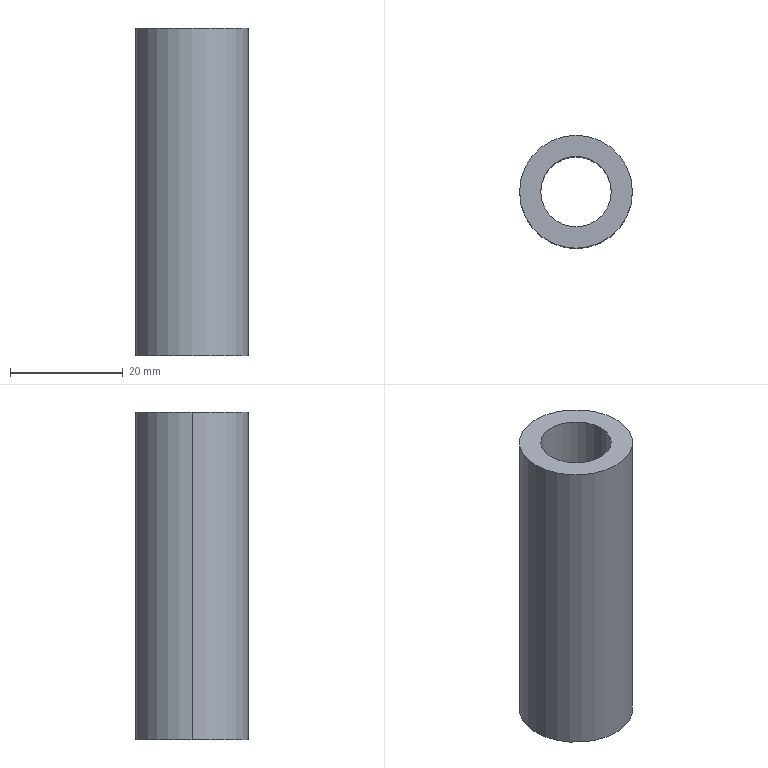Part | STEP file | X77-08309 | 1 solid | 6 faces | box 20 x 20 x 58 mm | volume 11104 mm3 | cylinder 4 | plane 2 | commonest cylinder face diameters 12.5 x2 20 x2
STEP:
#1=CARTESIAN_POINT('',(-36.25,627.253,58.));
#2=VERTEX_POINT('',#1);
#3=CARTESIAN_POINT('',(-23.75,627.253,58.));
#4=VERTEX_POINT('',#3);
#5=CARTESIAN_POINT('',(-30.,627.253,58.));
#6=DIRECTION('',(0.,0.,1.));
#7=DIRECTION('',(1.,0.,0.));
#8=AXIS2_PLACEMENT_3D('',#5,#6,#7);
#9=CIRCLE('',#8,6.25);
#10=EDGE_CURVE('',#2,#4,#9,.T.);
#11=ORIENTED_EDGE('',*,*,#10,.T.);
#12=CARTESIAN_POINT('',(-23.75,627.253,0.));
#13=VERTEX_POINT('',#12);
#14=CARTESIAN_POINT('',(-23.75,627.253,58.));
#15=DIRECTION('',(0.,0.,-1.));
#16=VECTOR('',#15,1000.);
#17=LINE('',#14,#16);
#18=EDGE_CURVE('',#4,#13,#17,.T.);
#19=ORIENTED_EDGE('',*,*,#18,.T.);
#20=CARTESIAN_POINT('',(-36.25,627.253,0.));
#21=VERTEX_POINT('',#20);
#22=CARTESIAN_POINT('',(-30.,627.253,0.));
#23=DIRECTION('',(0.,0.,1.));
#24=DIRECTION('',(1.,0.,0.));
#25=AXIS2_PLACEMENT_3D('',#22,#23,#24);
#26=CIRCLE('',#25,6.25);
#27=EDGE_CURVE('',#21,#13,#26,.T.);
#28=ORIENTED_EDGE('',*,*,#27,.F.);
#29=CARTESIAN_POINT('',(-36.25,627.253,58.));
#30=DIRECTION('',(0.,0.,-1.));
#31=VECTOR('',#30,1000.);
#32=LINE('',#29,#31);
#33=EDGE_CURVE('',#2,#21,#32,.T.);
#34=ORIENTED_EDGE('',*,*,#33,.F.);
#35=EDGE_LOOP('',(#11,#19,#28,#34));
#36=FACE_OUTER_BOUND('',#35,.T.);
#37=CARTESIAN_POINT('',(-30.,627.253,58.));
#38=DIRECTION('',(0.,0.,-1.));
#39=DIRECTION('',(-1.,0.,0.));
#40=AXIS2_PLACEMENT_3D('',#37,#38,#39);
#41=CYLINDRICAL_SURFACE('',#40,6.25);
#42=ADVANCED_FACE('',(#36),#41,.F.);
#43=CARTESIAN_POINT('',(-20.,627.253,58.));
#44=VERTEX_POINT('',#43);
#45=CARTESIAN_POINT('',(-40.,627.253,58.));
#46=VERTEX_POINT('',#45);
#47=CARTESIAN_POINT('',(-30.,627.253,58.));
#48=DIRECTION('',(0.,0.,1.));
#49=DIRECTION('',(1.,0.,0.));
#50=AXIS2_PLACEMENT_3D('',#47,#48,#49);
#51=CIRCLE('',#50,10.);
#52=EDGE_CURVE('',#44,#46,#51,.T.);
#53=ORIENTED_EDGE('',*,*,#52,.F.);
#54=CARTESIAN_POINT('',(-20.,627.253,0.));
#55=VERTEX_POINT('',#54);
#56=CARTESIAN_POINT('',(-20.,627.253,58.));
#57=DIRECTION('',(0.,0.,-1.));
#58=VECTOR('',#57,1000.);
#59=LINE('',#56,#58);
#60=EDGE_CURVE('',#44,#55,#59,.T.);
#61=ORIENTED_EDGE('',*,*,#60,.T.);
#62=CARTESIAN_POINT('',(-40.,627.253,0.));
#63=VERTEX_POINT('',#62);
#64=CARTESIAN_POINT('',(-30.,627.253,0.));
#65=DIRECTION('',(0.,0.,1.));
#66=DIRECTION('',(1.,0.,0.));
#67=AXIS2_PLACEMENT_3D('',#64,#65,#66);
#68=CIRCLE('',#67,10.);
#69=EDGE_CURVE('',#55,#63,#68,.T.);
#70=ORIENTED_EDGE('',*,*,#69,.T.);
#71=CARTESIAN_POINT('',(-40.,627.253,58.));
#72=DIRECTION('',(0.,0.,-1.));
#73=VECTOR('',#72,1000.);
#74=LINE('',#71,#73);
#75=EDGE_CURVE('',#46,#63,#74,.T.);
#76=ORIENTED_EDGE('',*,*,#75,.F.);
#77=EDGE_LOOP('',(#53,#61,#70,#76));
#78=FACE_OUTER_BOUND('',#77,.T.);
#79=CARTESIAN_POINT('',(-30.,627.253,58.));
#80=DIRECTION('',(0.,0.,-1.));
#81=DIRECTION('',(-1.,0.,0.));
#82=AXIS2_PLACEMENT_3D('',#79,#80,#81);
#83=CYLINDRICAL_SURFACE('',#82,10.);
#84=ADVANCED_FACE('',(#78),#83,.T.);
#85=CARTESIAN_POINT('',(-30.,627.253,58.));
#86=DIRECTION('',(0.,0.,1.));
#87=DIRECTION('',(1.,0.,0.));
#88=AXIS2_PLACEMENT_3D('',#85,#86,#87);
#89=CIRCLE('',#88,10.);
#90=EDGE_CURVE('',#46,#44,#89,.T.);
#91=ORIENTED_EDGE('',*,*,#90,.T.);
#92=ORIENTED_EDGE('',*,*,#52,.T.);
#93=EDGE_LOOP('',(#91,#92));
#94=FACE_OUTER_BOUND('',#93,.T.);
#95=ORIENTED_EDGE('',*,*,#10,.F.);
#96=CARTESIAN_POINT('',(-30.,627.253,58.));
#97=DIRECTION('',(0.,0.,1.));
#98=DIRECTION('',(1.,0.,0.));
#99=AXIS2_PLACEMENT_3D('',#96,#97,#98);
#100=CIRCLE('',#99,6.25);
#101=EDGE_CURVE('',#4,#2,#100,.T.);
#102=ORIENTED_EDGE('',*,*,#101,.F.);
#103=EDGE_LOOP('',(#95,#102));
#104=FACE_BOUND('',#103,.T.);
#105=CARTESIAN_POINT('',(-30.,627.253,58.));
#106=DIRECTION('',(0.,0.,1.));
#107=DIRECTION('',(1.,0.,0.));
#108=AXIS2_PLACEMENT_3D('',#105,#106,#107);
#109=PLANE('',#108);
#110=ADVANCED_FACE('',(#94,#104),#109,.T.);
#111=CARTESIAN_POINT('',(-30.,627.253,0.));
#112=DIRECTION('',(0.,0.,1.));
#113=DIRECTION('',(1.,0.,0.));
#114=AXIS2_PLACEMENT_3D('',#111,#112,#113);
#115=CIRCLE('',#114,10.);
#116=EDGE_CURVE('',#63,#55,#115,.T.);
#117=ORIENTED_EDGE('',*,*,#116,.F.);
#118=ORIENTED_EDGE('',*,*,#69,.F.);
#119=EDGE_LOOP('',(#117,#118));
#120=FACE_OUTER_BOUND('',#119,.T.);
#121=ORIENTED_EDGE('',*,*,#27,.T.);
#122=CARTESIAN_POINT('',(-30.,627.253,0.));
#123=DIRECTION('',(0.,0.,1.));
#124=DIRECTION('',(1.,0.,0.));
#125=AXIS2_PLACEMENT_3D('',#122,#123,#124);
#126=CIRCLE('',#125,6.25);
#127=EDGE_CURVE('',#13,#21,#126,.T.);
#128=ORIENTED_EDGE('',*,*,#127,.T.);
#129=EDGE_LOOP('',(#121,#128));
#130=FACE_BOUND('',#129,.T.);
#131=CARTESIAN_POINT('',(-30.,627.253,0.));
#132=DIRECTION('',(0.,0.,1.));
#133=DIRECTION('',(1.,0.,0.));
#134=AXIS2_PLACEMENT_3D('',#131,#132,#133);
#135=PLANE('',#134);
#136=ADVANCED_FACE('',(#120,#130),#135,.F.);
#137=ORIENTED_EDGE('',*,*,#60,.F.);
#138=ORIENTED_EDGE('',*,*,#90,.F.);
#139=ORIENTED_EDGE('',*,*,#75,.T.);
#140=ORIENTED_EDGE('',*,*,#116,.T.);
#141=EDGE_LOOP('',(#137,#138,#139,#140));
#142=FACE_OUTER_BOUND('',#141,.T.);
#143=CARTESIAN_POINT('',(-30.,627.253,58.));
#144=DIRECTION('',(0.,0.,-1.));
#145=DIRECTION('',(-1.,0.,0.));
#146=AXIS2_PLACEMENT_3D('',#143,#144,#145);
#147=CYLINDRICAL_SURFACE('',#146,10.);
#148=ADVANCED_FACE('',(#142),#147,.T.);
#149=ORIENTED_EDGE('',*,*,#18,.F.);
#150=ORIENTED_EDGE('',*,*,#101,.T.);
#151=ORIENTED_EDGE('',*,*,#33,.T.);
#152=ORIENTED_EDGE('',*,*,#127,.F.);
#153=EDGE_LOOP('',(#149,#150,#151,#152));
#154=FACE_OUTER_BOUND('',#153,.T.);
#155=CARTESIAN_POINT('',(-30.,627.253,58.));
#156=DIRECTION('',(0.,0.,-1.));
#157=DIRECTION('',(-1.,0.,0.));
#158=AXIS2_PLACEMENT_3D('',#155,#156,#157);
#159=CYLINDRICAL_SURFACE('',#158,6.25);
#160=ADVANCED_FACE('',(#154),#159,.F.);
#161=CLOSED_SHELL('',(#42,#84,#110,#136,#148,#160));
#162=MANIFOLD_SOLID_BREP('',#161);
#163=CARTESIAN_POINT('',(0.,0.,0.));
#164=DIRECTION('',(0.,0.,1.));
#165=DIRECTION('',(1.,0.,0.));
#166=AXIS2_PLACEMENT_3D('',#163,#164,#165);
#167=(LENGTH_UNIT()NAMED_UNIT(*)SI_UNIT(.MILLI.,.METRE.));
#168=UNCERTAINTY_MEASURE_WITH_UNIT(LENGTH_MEASURE(0.00001),#167,'','');
#169=(NAMED_UNIT(*)PLANE_ANGLE_UNIT()SI_UNIT($,.RADIAN.));
#170=(NAMED_UNIT(*)SI_UNIT($,.STERADIAN.)SOLID_ANGLE_UNIT());
#171=(GEOMETRIC_REPRESENTATION_CONTEXT(3)GLOBAL_UNCERTAINTY_ASSIGNED_CONTEXT((#168))GLOBAL_UNIT_ASSIGNED_CONTEXT((#167,#169,#170))REPRESENTATION_CONTEXT('',''));
#172=ADVANCED_BREP_SHAPE_REPRESENTATION('',(#162,#166),#171);